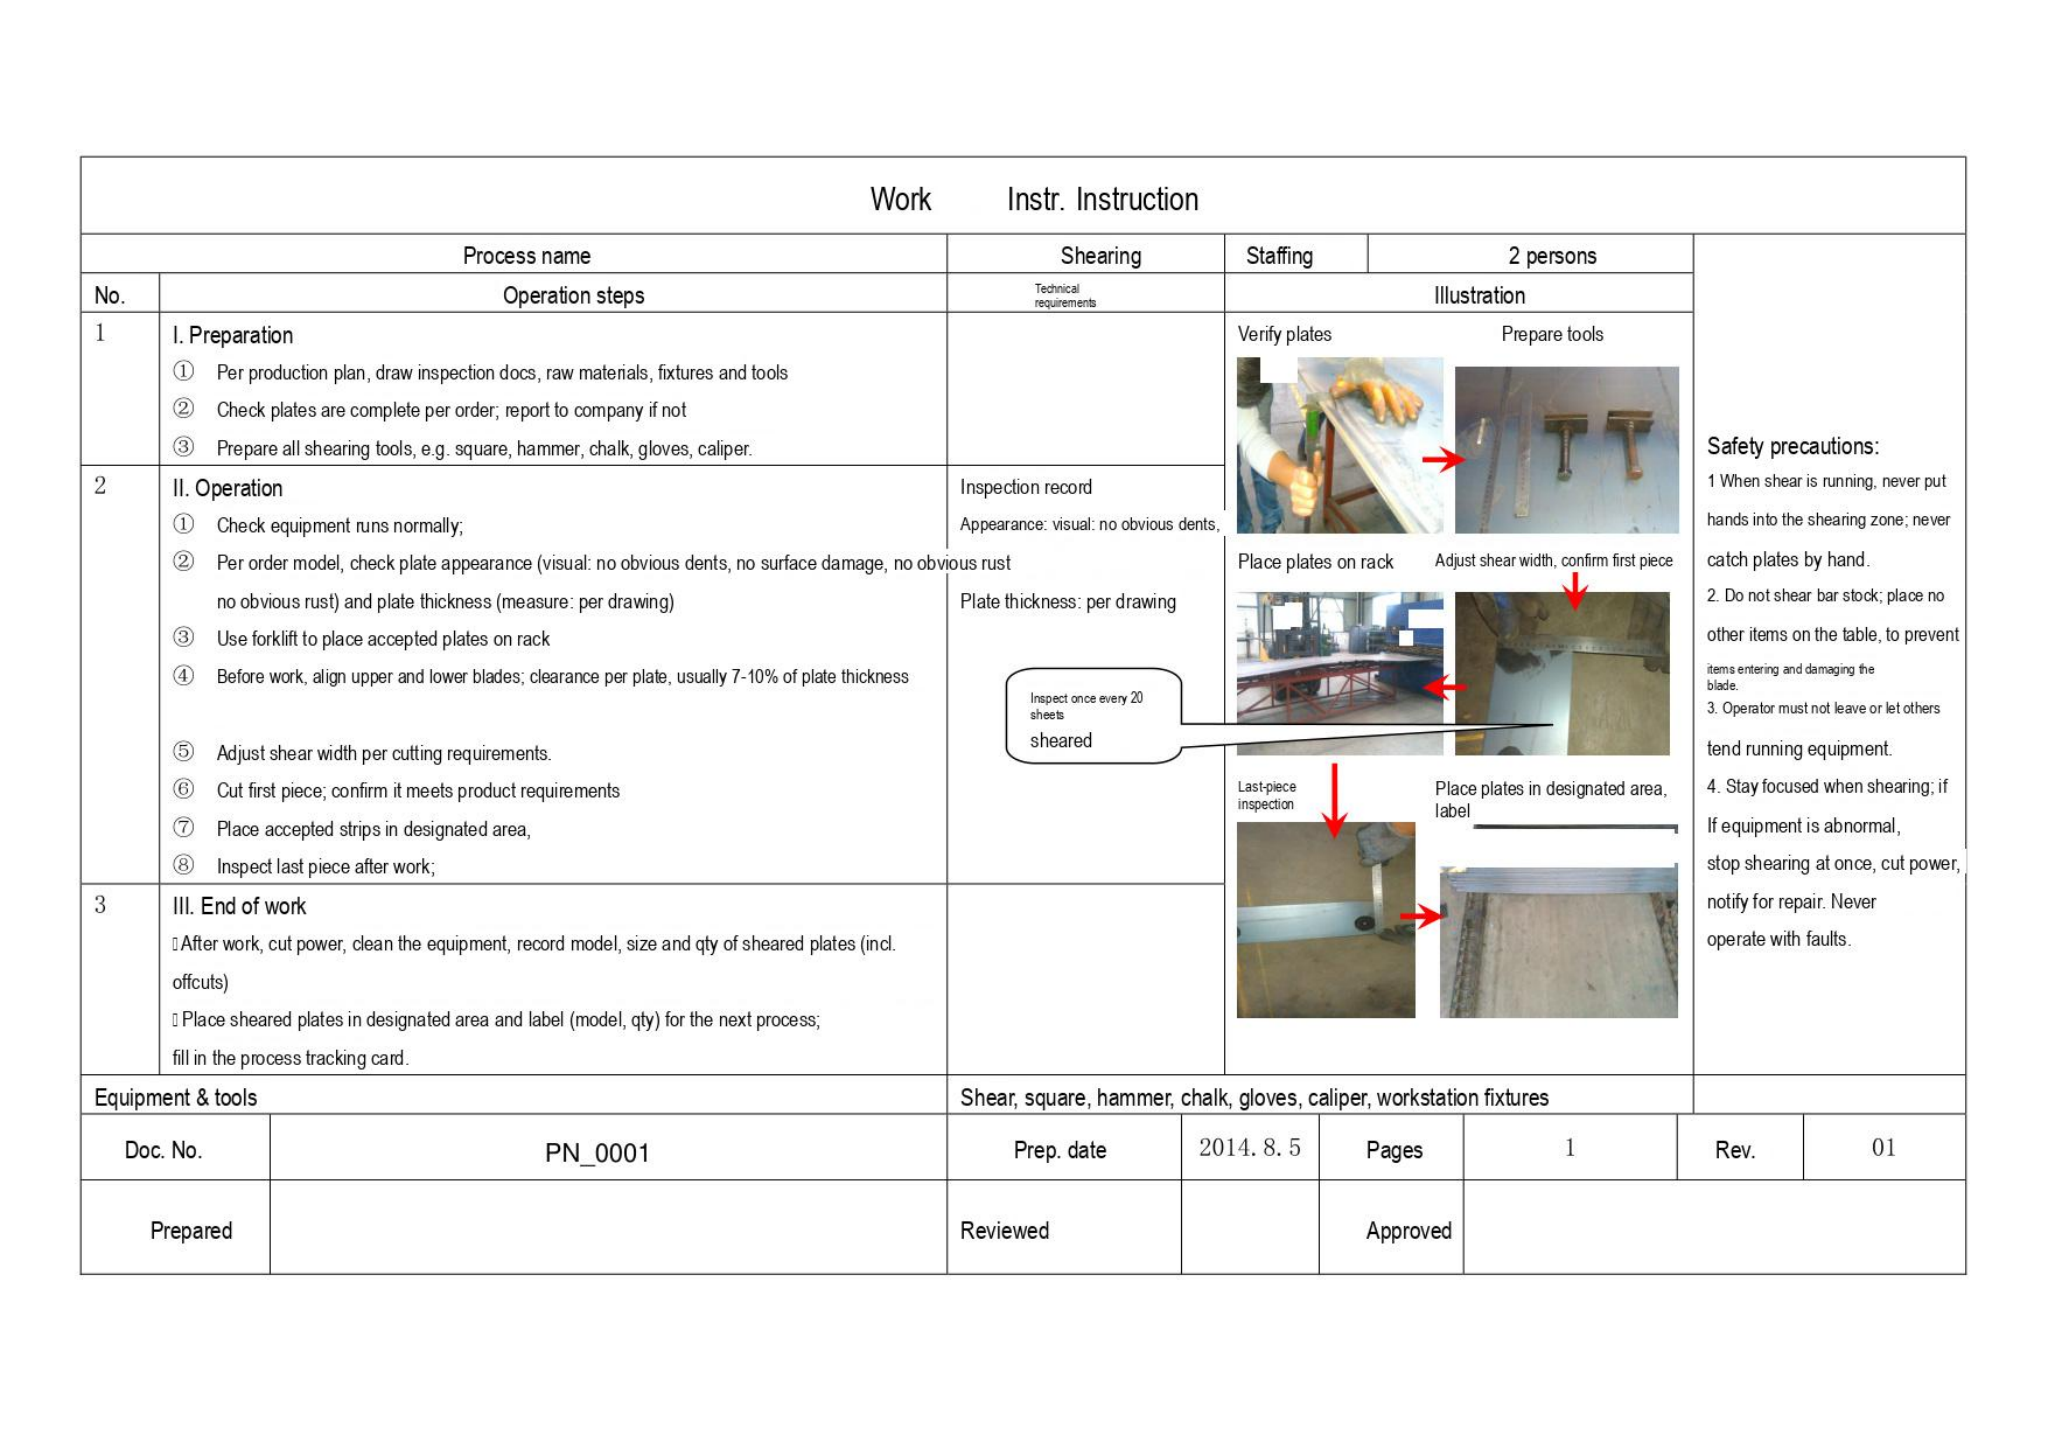# Work Instr. Instruction

| | Process name | Shearing | Staffing | 2 persons |
|---|---|---|---|---|

| No. | Operation steps | Technical requirements | Illustration | |
|---|---|---|---|---|
| 1 | I. Preparation<br>① Per production plan, draw inspection docs, raw materials, fixtures and tools<br>② Check plates are complete per order; report to company if not<br>③ Prepare all shearing tools, e.g. square, hammer, chalk, gloves, caliper. | | Verify plates<br>Prepare tools | Safety precautions:<br>1 When shear is running, never put hands into the shearing zone; never catch plates by hand.<br>2. Do not shear bar stock; place no other items on the table, to prevent items entering and damaging the blade.<br>3. Operator must not leave or let others tend running equipment.<br>4. Stay focused when shearing; if If equipment is abnormal, stop shearing at once, cut power, notify for repair. Never operate with faults. |
| 2 | II. Operation<br>① Check equipment runs normally;<br>② Per order model, check plate appearance (visual: no obvious dents, no surface damage, no obvious rust no obvious rust) and plate thickness (measure: per drawing)<br>③ Use forklift to place accepted plates on rack<br>④ Before work, align upper and lower blades; clearance per plate, usually 7-10% of plate thickness<br>⑤ Adjust shear width per cutting requirements.<br>⑥ Cut first piece; confirm it meets product requirements<br>⑦ Place accepted strips in designated area,<br>⑧ Inspect last piece after work; | Inspection record<br>Appearance: visual: no obvious dents,<br>Plate thickness: per drawing<br>Inspect once every 20 sheets sheared | Place plates on rack<br>Adjust shear width, confirm first piece<br>Last-piece inspection<br>Place plates in designated area, label | |
| 3 | III. End of work<br>After work, cut power, clean the equipment, record model, size and qty of sheared plates (incl. offcuts)<br>Place sheared plates in designated area and label (model, qty) for the next process; fill in the process tracking card. | | | |

| Equipment & tools | Shear, square, hammer, chalk, gloves, caliper, workstation fixtures |
|---|---|

| Doc. No. | PN_0001 | Prep. date | 2014. 8. 5 | Pages | 1 | Rev. | 01 |
|---|---|---|---|---|---|---|---|
| Prepared | | Reviewed | | Approved | | | |